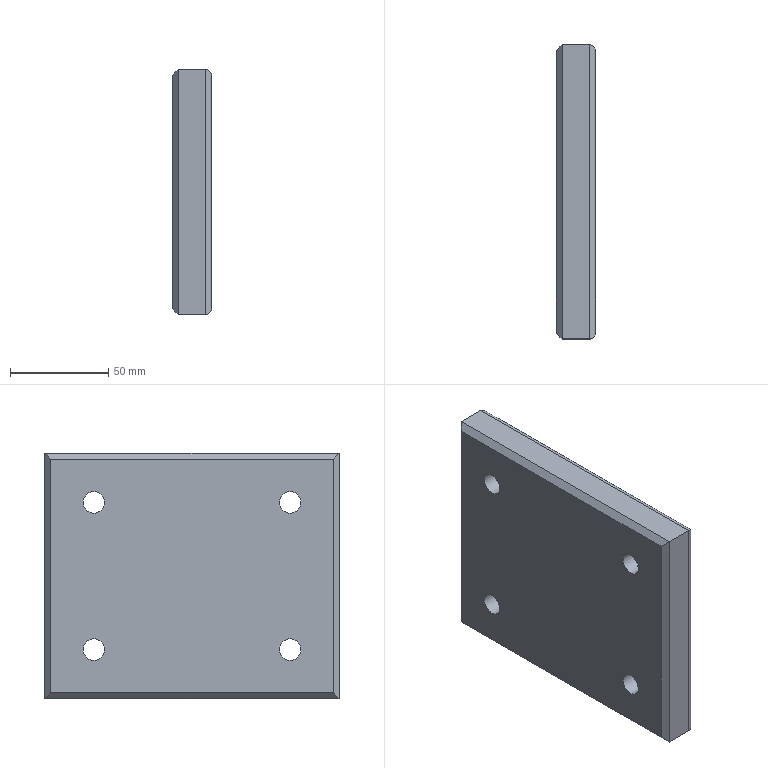Part | NX | features solid 2 | 1 solid | 26 faces | box 20 x 150 x 125 mm | volume 356923 mm3 | plane 14 | cylinder 12 | commonest cylinder face diameters 6 x4 11 x4 17.5 x4
STEP:
#1=CARTESIAN_POINT('',(803.,75.,-130.));
#2=VERTEX_POINT('',#1);
#3=CARTESIAN_POINT('',(817.,75.,-130.));
#4=VERTEX_POINT('',#3);
#5=CARTESIAN_POINT('',(800.,75.,-130.));
#6=DIRECTION('',(1.,0.,0.));
#7=VECTOR('',#6,1000.);
#8=LINE('',#5,#7);
#9=EDGE_CURVE('',#2,#4,#8,.T.);
#10=ORIENTED_EDGE('',*,*,#9,.T.);
#11=CARTESIAN_POINT('',(817.,-75.,-130.));
#12=VERTEX_POINT('',#11);
#13=CARTESIAN_POINT('',(817.,50.,-130.));
#14=DIRECTION('',(0.,1.,0.));
#15=VECTOR('',#14,1000.);
#16=LINE('',#13,#15);
#17=EDGE_CURVE('',#12,#4,#16,.T.);
#18=ORIENTED_EDGE('',*,*,#17,.F.);
#19=CARTESIAN_POINT('',(803.,-75.,-130.));
#20=VERTEX_POINT('',#19);
#21=CARTESIAN_POINT('',(800.,-75.,-130.));
#22=DIRECTION('',(1.,0.,0.));
#23=VECTOR('',#22,1000.);
#24=LINE('',#21,#23);
#25=EDGE_CURVE('',#20,#12,#24,.T.);
#26=ORIENTED_EDGE('',*,*,#25,.F.);
#27=CARTESIAN_POINT('',(803.,-50.,-130.));
#28=DIRECTION('',(0.,-1.,0.));
#29=VECTOR('',#28,1000.);
#30=LINE('',#27,#29);
#31=EDGE_CURVE('',#2,#20,#30,.T.);
#32=ORIENTED_EDGE('',*,*,#31,.F.);
#33=EDGE_LOOP('',(#10,#18,#26,#32));
#34=FACE_BOUND('',#33,.T.);
#35=CARTESIAN_POINT('',(800.,-50.,-130.));
#36=DIRECTION('',(0.,0.,1.));
#37=DIRECTION('',(0.,-1.,0.));
#38=AXIS2_PLACEMENT_3D('',#35,#36,#37);
#39=PLANE('',#38);
#40=ADVANCED_FACE('',(#34),#39,.F.);
#41=CARTESIAN_POINT('',(803.,75.,-5.));
#42=VERTEX_POINT('',#41);
#43=CARTESIAN_POINT('',(817.,75.,-5.));
#44=VERTEX_POINT('',#43);
#45=CARTESIAN_POINT('',(800.,75.,-5.));
#46=DIRECTION('',(1.,0.,0.));
#47=VECTOR('',#46,1000.);
#48=LINE('',#45,#47);
#49=EDGE_CURVE('',#42,#44,#48,.T.);
#50=ORIENTED_EDGE('',*,*,#49,.T.);
#51=CARTESIAN_POINT('',(817.,75.,-5.));
#52=DIRECTION('',(0.,0.,1.));
#53=VECTOR('',#52,1000.);
#54=LINE('',#51,#53);
#55=EDGE_CURVE('',#4,#44,#54,.T.);
#56=ORIENTED_EDGE('',*,*,#55,.F.);
#57=ORIENTED_EDGE('',*,*,#9,.F.);
#58=CARTESIAN_POINT('',(803.,75.,-105.));
#59=DIRECTION('',(0.,0.,-1.));
#60=VECTOR('',#59,1000.);
#61=LINE('',#58,#60);
#62=EDGE_CURVE('',#42,#2,#61,.T.);
#63=ORIENTED_EDGE('',*,*,#62,.F.);
#64=EDGE_LOOP('',(#50,#56,#57,#63));
#65=FACE_BOUND('',#64,.T.);
#66=CARTESIAN_POINT('',(800.,75.,-105.));
#67=DIRECTION('',(0.,-1.,0.));
#68=DIRECTION('',(-1.,0.,0.));
#69=AXIS2_PLACEMENT_3D('',#66,#67,#68);
#70=PLANE('',#69);
#71=ADVANCED_FACE('',(#65),#70,.F.);
#72=CARTESIAN_POINT('',(803.,-75.,-5.));
#73=VERTEX_POINT('',#72);
#74=CARTESIAN_POINT('',(817.,-75.,-5.));
#75=VERTEX_POINT('',#74);
#76=CARTESIAN_POINT('',(800.,-75.,-5.));
#77=DIRECTION('',(1.,0.,0.));
#78=VECTOR('',#77,1000.);
#79=LINE('',#76,#78);
#80=EDGE_CURVE('',#73,#75,#79,.T.);
#81=ORIENTED_EDGE('',*,*,#80,.T.);
#82=CARTESIAN_POINT('',(817.,-50.,-5.));
#83=DIRECTION('',(0.,-1.,0.));
#84=VECTOR('',#83,1000.);
#85=LINE('',#82,#84);
#86=EDGE_CURVE('',#44,#75,#85,.T.);
#87=ORIENTED_EDGE('',*,*,#86,.F.);
#88=ORIENTED_EDGE('',*,*,#49,.F.);
#89=CARTESIAN_POINT('',(803.,50.,-5.));
#90=DIRECTION('',(0.,1.,0.));
#91=VECTOR('',#90,1000.);
#92=LINE('',#89,#91);
#93=EDGE_CURVE('',#73,#42,#92,.T.);
#94=ORIENTED_EDGE('',*,*,#93,.F.);
#95=EDGE_LOOP('',(#81,#87,#88,#94));
#96=FACE_BOUND('',#95,.T.);
#97=CARTESIAN_POINT('',(800.,50.,-5.));
#98=DIRECTION('',(0.,0.,-1.));
#99=DIRECTION('',(-1.,0.,0.));
#100=AXIS2_PLACEMENT_3D('',#97,#98,#99);
#101=PLANE('',#100);
#102=ADVANCED_FACE('',(#96),#101,.F.);
#103=ORIENTED_EDGE('',*,*,#25,.T.);
#104=CARTESIAN_POINT('',(817.,-75.,-105.));
#105=DIRECTION('',(0.,0.,-1.));
#106=VECTOR('',#105,1000.);
#107=LINE('',#104,#106);
#108=EDGE_CURVE('',#75,#12,#107,.T.);
#109=ORIENTED_EDGE('',*,*,#108,.F.);
#110=ORIENTED_EDGE('',*,*,#80,.F.);
#111=CARTESIAN_POINT('',(803.,-75.,-5.));
#112=DIRECTION('',(0.,0.,1.));
#113=VECTOR('',#112,1000.);
#114=LINE('',#111,#113);
#115=EDGE_CURVE('',#20,#73,#114,.T.);
#116=ORIENTED_EDGE('',*,*,#115,.F.);
#117=EDGE_LOOP('',(#103,#109,#110,#116));
#118=FACE_BOUND('',#117,.T.);
#119=CARTESIAN_POINT('',(800.,-75.,-5.));
#120=DIRECTION('',(0.,1.,0.));
#121=DIRECTION('',(0.,0.,1.));
#122=AXIS2_PLACEMENT_3D('',#119,#120,#121);
#123=PLANE('',#122);
#124=ADVANCED_FACE('',(#118),#123,.F.);
#125=CARTESIAN_POINT('',(800.,72.,-127.));
#126=VERTEX_POINT('',#125);
#127=CARTESIAN_POINT('',(800.,72.,-8.));
#128=VERTEX_POINT('',#127);
#129=CARTESIAN_POINT('',(800.,72.,-105.));
#130=DIRECTION('',(0.,0.,1.));
#131=VECTOR('',#130,1000.);
#132=LINE('',#129,#131);
#133=EDGE_CURVE('',#126,#128,#132,.T.);
#134=ORIENTED_EDGE('',*,*,#133,.F.);
#135=CARTESIAN_POINT('',(800.,-72.,-127.));
#136=VERTEX_POINT('',#135);
#137=CARTESIAN_POINT('',(800.,-50.,-127.));
#138=DIRECTION('',(0.,1.,0.));
#139=VECTOR('',#138,1000.);
#140=LINE('',#137,#139);
#141=EDGE_CURVE('',#136,#126,#140,.T.);
#142=ORIENTED_EDGE('',*,*,#141,.F.);
#143=CARTESIAN_POINT('',(800.,-72.,-8.));
#144=VERTEX_POINT('',#143);
#145=CARTESIAN_POINT('',(800.,-72.,-105.));
#146=DIRECTION('',(0.,0.,-1.));
#147=VECTOR('',#146,1000.);
#148=LINE('',#145,#147);
#149=EDGE_CURVE('',#144,#136,#148,.T.);
#150=ORIENTED_EDGE('',*,*,#149,.F.);
#151=CARTESIAN_POINT('',(800.,-50.,-8.));
#152=DIRECTION('',(0.,-1.,0.));
#153=VECTOR('',#152,1000.);
#154=LINE('',#151,#153);
#155=EDGE_CURVE('',#128,#144,#154,.T.);
#156=ORIENTED_EDGE('',*,*,#155,.F.);
#157=EDGE_LOOP('',(#134,#142,#150,#156));
#158=FACE_BOUND('',#157,.T.);
#159=CARTESIAN_POINT('',(800.,50.,-35.5));
#160=VERTEX_POINT('',#159);
#161=CARTESIAN_POINT('',(800.,50.,-30.));
#162=DIRECTION('',(-1.,0.,0.));
#163=DIRECTION('',(0.,0.,-1.));
#164=AXIS2_PLACEMENT_3D('',#161,#162,#163);
#165=CIRCLE('',#164,5.5);
#166=EDGE_CURVE('',#160,#160,#165,.T.);
#167=ORIENTED_EDGE('',*,*,#166,.F.);
#168=EDGE_LOOP('',(#167));
#169=FACE_BOUND('',#168,.T.);
#170=CARTESIAN_POINT('',(800.,-50.,-35.5));
#171=VERTEX_POINT('',#170);
#172=CARTESIAN_POINT('',(800.,-50.,-30.));
#173=DIRECTION('',(-1.,0.,0.));
#174=DIRECTION('',(0.,0.,-1.));
#175=AXIS2_PLACEMENT_3D('',#172,#173,#174);
#176=CIRCLE('',#175,5.5);
#177=EDGE_CURVE('',#171,#171,#176,.T.);
#178=ORIENTED_EDGE('',*,*,#177,.F.);
#179=EDGE_LOOP('',(#178));
#180=FACE_BOUND('',#179,.T.);
#181=CARTESIAN_POINT('',(800.,50.,-110.5));
#182=VERTEX_POINT('',#181);
#183=CARTESIAN_POINT('',(800.,50.,-105.));
#184=DIRECTION('',(-1.,0.,0.));
#185=DIRECTION('',(0.,0.,-1.));
#186=AXIS2_PLACEMENT_3D('',#183,#184,#185);
#187=CIRCLE('',#186,5.5);
#188=EDGE_CURVE('',#182,#182,#187,.T.);
#189=ORIENTED_EDGE('',*,*,#188,.F.);
#190=EDGE_LOOP('',(#189));
#191=FACE_BOUND('',#190,.T.);
#192=CARTESIAN_POINT('',(800.,-50.,-110.5));
#193=VERTEX_POINT('',#192);
#194=CARTESIAN_POINT('',(800.,-50.,-105.));
#195=DIRECTION('',(-1.,0.,0.));
#196=DIRECTION('',(0.,0.,-1.));
#197=AXIS2_PLACEMENT_3D('',#194,#195,#196);
#198=CIRCLE('',#197,5.5);
#199=EDGE_CURVE('',#193,#193,#198,.T.);
#200=ORIENTED_EDGE('',*,*,#199,.F.);
#201=EDGE_LOOP('',(#200));
#202=FACE_BOUND('',#201,.T.);
#203=CARTESIAN_POINT('',(800.,-50.,-105.));
#204=DIRECTION('',(1.,0.,0.));
#205=DIRECTION('',(0.,0.,-1.));
#206=AXIS2_PLACEMENT_3D('',#203,#204,#205);
#207=PLANE('',#206);
#208=ADVANCED_FACE('',(#158,#169,#180,#191,#202),#207,.F.);
#209=CARTESIAN_POINT('',(820.,72.,-127.));
#210=VERTEX_POINT('',#209);
#211=CARTESIAN_POINT('',(820.,-72.,-127.));
#212=VERTEX_POINT('',#211);
#213=CARTESIAN_POINT('',(820.,-50.,-127.));
#214=DIRECTION('',(0.,1.,0.));
#215=VECTOR('',#214,1000.);
#216=LINE('',#213,#215);
#217=EDGE_CURVE('',#210,#212,#216,.F.);
#218=ORIENTED_EDGE('',*,*,#217,.F.);
#219=CARTESIAN_POINT('',(820.,72.,-8.));
#220=VERTEX_POINT('',#219);
#221=CARTESIAN_POINT('',(820.,72.,-105.));
#222=DIRECTION('',(0.,0.,1.));
#223=VECTOR('',#222,1000.);
#224=LINE('',#221,#223);
#225=EDGE_CURVE('',#220,#210,#224,.F.);
#226=ORIENTED_EDGE('',*,*,#225,.F.);
#227=CARTESIAN_POINT('',(820.,-72.,-8.));
#228=VERTEX_POINT('',#227);
#229=CARTESIAN_POINT('',(820.,50.,-8.));
#230=DIRECTION('',(0.,-1.,0.));
#231=VECTOR('',#230,1000.);
#232=LINE('',#229,#231);
#233=EDGE_CURVE('',#228,#220,#232,.F.);
#234=ORIENTED_EDGE('',*,*,#233,.F.);
#235=CARTESIAN_POINT('',(820.,-72.,-5.));
#236=DIRECTION('',(0.,0.,-1.));
#237=VECTOR('',#236,1000.);
#238=LINE('',#235,#237);
#239=EDGE_CURVE('',#212,#228,#238,.F.);
#240=ORIENTED_EDGE('',*,*,#239,.F.);
#241=EDGE_LOOP('',(#218,#226,#234,#240));
#242=FACE_BOUND('',#241,.T.);
#243=CARTESIAN_POINT('',(820.,50.,-21.25));
#244=VERTEX_POINT('',#243);
#245=CARTESIAN_POINT('',(820.,50.,-30.));
#246=DIRECTION('',(1.,0.,0.));
#247=DIRECTION('',(0.,0.,1.));
#248=AXIS2_PLACEMENT_3D('',#245,#246,#247);
#249=CIRCLE('',#248,8.75);
#250=EDGE_CURVE('',#244,#244,#249,.T.);
#251=ORIENTED_EDGE('',*,*,#250,.F.);
#252=EDGE_LOOP('',(#251));
#253=FACE_BOUND('',#252,.T.);
#254=CARTESIAN_POINT('',(820.,-50.,-21.25));
#255=VERTEX_POINT('',#254);
#256=CARTESIAN_POINT('',(820.,-50.,-30.));
#257=DIRECTION('',(1.,0.,0.));
#258=DIRECTION('',(0.,0.,1.));
#259=AXIS2_PLACEMENT_3D('',#256,#257,#258);
#260=CIRCLE('',#259,8.75);
#261=EDGE_CURVE('',#255,#255,#260,.T.);
#262=ORIENTED_EDGE('',*,*,#261,.F.);
#263=EDGE_LOOP('',(#262));
#264=FACE_BOUND('',#263,.T.);
#265=CARTESIAN_POINT('',(820.,50.,-96.25));
#266=VERTEX_POINT('',#265);
#267=CARTESIAN_POINT('',(820.,50.,-105.));
#268=DIRECTION('',(1.,0.,0.));
#269=DIRECTION('',(0.,0.,1.));
#270=AXIS2_PLACEMENT_3D('',#267,#268,#269);
#271=CIRCLE('',#270,8.75);
#272=EDGE_CURVE('',#266,#266,#271,.T.);
#273=ORIENTED_EDGE('',*,*,#272,.F.);
#274=EDGE_LOOP('',(#273));
#275=FACE_BOUND('',#274,.T.);
#276=CARTESIAN_POINT('',(820.,-50.,-96.25));
#277=VERTEX_POINT('',#276);
#278=CARTESIAN_POINT('',(820.,-50.,-105.));
#279=DIRECTION('',(1.,0.,0.));
#280=DIRECTION('',(0.,0.,1.));
#281=AXIS2_PLACEMENT_3D('',#278,#279,#280);
#282=CIRCLE('',#281,8.75);
#283=EDGE_CURVE('',#277,#277,#282,.T.);
#284=ORIENTED_EDGE('',*,*,#283,.F.);
#285=EDGE_LOOP('',(#284));
#286=FACE_BOUND('',#285,.T.);
#287=CARTESIAN_POINT('',(820.,-50.,-105.));
#288=DIRECTION('',(1.,0.,0.));
#289=DIRECTION('',(0.,0.,-1.));
#290=AXIS2_PLACEMENT_3D('',#287,#288,#289);
#291=PLANE('',#290);
#292=ADVANCED_FACE('',(#242,#253,#264,#275,#286),#291,.T.);
#293=CARTESIAN_POINT('',(808.,-50.,-99.5));
#294=VERTEX_POINT('',#293);
#295=CARTESIAN_POINT('',(808.,-50.,-105.));
#296=DIRECTION('',(1.,0.,0.));
#297=DIRECTION('',(0.,0.,1.));
#298=AXIS2_PLACEMENT_3D('',#295,#296,#297);
#299=CIRCLE('',#298,5.5);
#300=EDGE_CURVE('',#294,#294,#299,.T.);
#301=ORIENTED_EDGE('',*,*,#300,.T.);
#302=EDGE_LOOP('',(#301));
#303=FACE_BOUND('',#302,.T.);
#304=ORIENTED_EDGE('',*,*,#199,.T.);
#305=EDGE_LOOP('',(#304));
#306=FACE_BOUND('',#305,.T.);
#307=CARTESIAN_POINT('',(770.,-50.,-105.));
#308=DIRECTION('',(-1.,0.,0.));
#309=DIRECTION('',(0.,0.,1.));
#310=AXIS2_PLACEMENT_3D('',#307,#308,#309);
#311=CYLINDRICAL_SURFACE('',#310,5.5);
#312=ADVANCED_FACE('',(#303,#306),#311,.F.);
#313=ORIENTED_EDGE('',*,*,#300,.F.);
#314=EDGE_LOOP('',(#313));
#315=FACE_BOUND('',#314,.T.);
#316=CARTESIAN_POINT('',(808.,-50.,-96.25));
#317=VERTEX_POINT('',#316);
#318=CARTESIAN_POINT('',(808.,-50.,-105.));
#319=DIRECTION('',(1.,0.,0.));
#320=DIRECTION('',(0.,0.,1.));
#321=AXIS2_PLACEMENT_3D('',#318,#319,#320);
#322=CIRCLE('',#321,8.75);
#323=EDGE_CURVE('',#317,#317,#322,.T.);
#324=ORIENTED_EDGE('',*,*,#323,.T.);
#325=EDGE_LOOP('',(#324));
#326=FACE_BOUND('',#325,.T.);
#327=CARTESIAN_POINT('',(808.,-50.,-105.));
#328=DIRECTION('',(-1.,0.,0.));
#329=DIRECTION('',(0.,0.,1.));
#330=AXIS2_PLACEMENT_3D('',#327,#328,#329);
#331=PLANE('',#330);
#332=ADVANCED_FACE('',(#315,#326),#331,.F.);
#333=ORIENTED_EDGE('',*,*,#323,.F.);
#334=EDGE_LOOP('',(#333));
#335=FACE_BOUND('',#334,.T.);
#336=ORIENTED_EDGE('',*,*,#283,.T.);
#337=EDGE_LOOP('',(#336));
#338=FACE_BOUND('',#337,.T.);
#339=CARTESIAN_POINT('',(820.,-50.,-105.));
#340=DIRECTION('',(-1.,0.,0.));
#341=DIRECTION('',(0.,0.,1.));
#342=AXIS2_PLACEMENT_3D('',#339,#340,#341);
#343=CYLINDRICAL_SURFACE('',#342,8.75);
#344=ADVANCED_FACE('',(#335,#338),#343,.F.);
#345=CARTESIAN_POINT('',(808.,50.,-99.5));
#346=VERTEX_POINT('',#345);
#347=CARTESIAN_POINT('',(808.,50.,-105.));
#348=DIRECTION('',(1.,0.,0.));
#349=DIRECTION('',(0.,0.,1.));
#350=AXIS2_PLACEMENT_3D('',#347,#348,#349);
#351=CIRCLE('',#350,5.5);
#352=EDGE_CURVE('',#346,#346,#351,.T.);
#353=ORIENTED_EDGE('',*,*,#352,.T.);
#354=EDGE_LOOP('',(#353));
#355=FACE_BOUND('',#354,.T.);
#356=ORIENTED_EDGE('',*,*,#188,.T.);
#357=EDGE_LOOP('',(#356));
#358=FACE_BOUND('',#357,.T.);
#359=CARTESIAN_POINT('',(770.,50.,-105.));
#360=DIRECTION('',(-1.,0.,0.));
#361=DIRECTION('',(0.,0.,1.));
#362=AXIS2_PLACEMENT_3D('',#359,#360,#361);
#363=CYLINDRICAL_SURFACE('',#362,5.5);
#364=ADVANCED_FACE('',(#355,#358),#363,.F.);
#365=ORIENTED_EDGE('',*,*,#352,.F.);
#366=EDGE_LOOP('',(#365));
#367=FACE_BOUND('',#366,.T.);
#368=CARTESIAN_POINT('',(808.,50.,-96.25));
#369=VERTEX_POINT('',#368);
#370=CARTESIAN_POINT('',(808.,50.,-105.));
#371=DIRECTION('',(1.,0.,0.));
#372=DIRECTION('',(0.,0.,1.));
#373=AXIS2_PLACEMENT_3D('',#370,#371,#372);
#374=CIRCLE('',#373,8.75);
#375=EDGE_CURVE('',#369,#369,#374,.T.);
#376=ORIENTED_EDGE('',*,*,#375,.T.);
#377=EDGE_LOOP('',(#376));
#378=FACE_BOUND('',#377,.T.);
#379=CARTESIAN_POINT('',(808.,50.,-105.));
#380=DIRECTION('',(-1.,0.,0.));
#381=DIRECTION('',(0.,0.,1.));
#382=AXIS2_PLACEMENT_3D('',#379,#380,#381);
#383=PLANE('',#382);
#384=ADVANCED_FACE('',(#367,#378),#383,.F.);
#385=ORIENTED_EDGE('',*,*,#375,.F.);
#386=EDGE_LOOP('',(#385));
#387=FACE_BOUND('',#386,.T.);
#388=ORIENTED_EDGE('',*,*,#272,.T.);
#389=EDGE_LOOP('',(#388));
#390=FACE_BOUND('',#389,.T.);
#391=CARTESIAN_POINT('',(820.,50.,-105.));
#392=DIRECTION('',(-1.,0.,0.));
#393=DIRECTION('',(0.,0.,1.));
#394=AXIS2_PLACEMENT_3D('',#391,#392,#393);
#395=CYLINDRICAL_SURFACE('',#394,8.75);
#396=ADVANCED_FACE('',(#387,#390),#395,.F.);
#397=CARTESIAN_POINT('',(808.,-50.,-24.5));
#398=VERTEX_POINT('',#397);
#399=CARTESIAN_POINT('',(808.,-50.,-30.));
#400=DIRECTION('',(1.,0.,0.));
#401=DIRECTION('',(0.,0.,1.));
#402=AXIS2_PLACEMENT_3D('',#399,#400,#401);
#403=CIRCLE('',#402,5.5);
#404=EDGE_CURVE('',#398,#398,#403,.T.);
#405=ORIENTED_EDGE('',*,*,#404,.T.);
#406=EDGE_LOOP('',(#405));
#407=FACE_BOUND('',#406,.T.);
#408=ORIENTED_EDGE('',*,*,#177,.T.);
#409=EDGE_LOOP('',(#408));
#410=FACE_BOUND('',#409,.T.);
#411=CARTESIAN_POINT('',(770.,-50.,-30.));
#412=DIRECTION('',(-1.,0.,0.));
#413=DIRECTION('',(0.,0.,1.));
#414=AXIS2_PLACEMENT_3D('',#411,#412,#413);
#415=CYLINDRICAL_SURFACE('',#414,5.5);
#416=ADVANCED_FACE('',(#407,#410),#415,.F.);
#417=ORIENTED_EDGE('',*,*,#404,.F.);
#418=EDGE_LOOP('',(#417));
#419=FACE_BOUND('',#418,.T.);
#420=CARTESIAN_POINT('',(808.,-50.,-21.25));
#421=VERTEX_POINT('',#420);
#422=CARTESIAN_POINT('',(808.,-50.,-30.));
#423=DIRECTION('',(1.,0.,0.));
#424=DIRECTION('',(0.,0.,1.));
#425=AXIS2_PLACEMENT_3D('',#422,#423,#424);
#426=CIRCLE('',#425,8.75);
#427=EDGE_CURVE('',#421,#421,#426,.T.);
#428=ORIENTED_EDGE('',*,*,#427,.T.);
#429=EDGE_LOOP('',(#428));
#430=FACE_BOUND('',#429,.T.);
#431=CARTESIAN_POINT('',(808.,-50.,-30.));
#432=DIRECTION('',(-1.,0.,0.));
#433=DIRECTION('',(0.,0.,1.));
#434=AXIS2_PLACEMENT_3D('',#431,#432,#433);
#435=PLANE('',#434);
#436=ADVANCED_FACE('',(#419,#430),#435,.F.);
#437=ORIENTED_EDGE('',*,*,#427,.F.);
#438=EDGE_LOOP('',(#437));
#439=FACE_BOUND('',#438,.T.);
#440=ORIENTED_EDGE('',*,*,#261,.T.);
#441=EDGE_LOOP('',(#440));
#442=FACE_BOUND('',#441,.T.);
#443=CARTESIAN_POINT('',(820.,-50.,-30.));
#444=DIRECTION('',(-1.,0.,0.));
#445=DIRECTION('',(0.,0.,1.));
#446=AXIS2_PLACEMENT_3D('',#443,#444,#445);
#447=CYLINDRICAL_SURFACE('',#446,8.75);
#448=ADVANCED_FACE('',(#439,#442),#447,.F.);
#449=CARTESIAN_POINT('',(808.,50.,-24.5));
#450=VERTEX_POINT('',#449);
#451=CARTESIAN_POINT('',(808.,50.,-30.));
#452=DIRECTION('',(1.,0.,0.));
#453=DIRECTION('',(0.,0.,1.));
#454=AXIS2_PLACEMENT_3D('',#451,#452,#453);
#455=CIRCLE('',#454,5.5);
#456=EDGE_CURVE('',#450,#450,#455,.T.);
#457=ORIENTED_EDGE('',*,*,#456,.T.);
#458=EDGE_LOOP('',(#457));
#459=FACE_BOUND('',#458,.T.);
#460=ORIENTED_EDGE('',*,*,#166,.T.);
#461=EDGE_LOOP('',(#460));
#462=FACE_BOUND('',#461,.T.);
#463=CARTESIAN_POINT('',(770.,50.,-30.));
#464=DIRECTION('',(-1.,0.,0.));
#465=DIRECTION('',(0.,0.,1.));
#466=AXIS2_PLACEMENT_3D('',#463,#464,#465);
#467=CYLINDRICAL_SURFACE('',#466,5.5);
#468=ADVANCED_FACE('',(#459,#462),#467,.F.);
#469=ORIENTED_EDGE('',*,*,#456,.F.);
#470=EDGE_LOOP('',(#469));
#471=FACE_BOUND('',#470,.T.);
#472=CARTESIAN_POINT('',(808.,50.,-21.25));
#473=VERTEX_POINT('',#472);
#474=CARTESIAN_POINT('',(808.,50.,-30.));
#475=DIRECTION('',(1.,0.,0.));
#476=DIRECTION('',(0.,0.,1.));
#477=AXIS2_PLACEMENT_3D('',#474,#475,#476);
#478=CIRCLE('',#477,8.75);
#479=EDGE_CURVE('',#473,#473,#478,.T.);
#480=ORIENTED_EDGE('',*,*,#479,.T.);
#481=EDGE_LOOP('',(#480));
#482=FACE_BOUND('',#481,.T.);
#483=CARTESIAN_POINT('',(808.,50.,-30.));
#484=DIRECTION('',(-1.,0.,0.));
#485=DIRECTION('',(0.,0.,1.));
#486=AXIS2_PLACEMENT_3D('',#483,#484,#485);
#487=PLANE('',#486);
#488=ADVANCED_FACE('',(#471,#482),#487,.F.);
#489=ORIENTED_EDGE('',*,*,#479,.F.);
#490=EDGE_LOOP('',(#489));
#491=FACE_BOUND('',#490,.T.);
#492=ORIENTED_EDGE('',*,*,#250,.T.);
#493=EDGE_LOOP('',(#492));
#494=FACE_BOUND('',#493,.T.);
#495=CARTESIAN_POINT('',(820.,50.,-30.));
#496=DIRECTION('',(-1.,0.,0.));
#497=DIRECTION('',(0.,0.,1.));
#498=AXIS2_PLACEMENT_3D('',#495,#496,#497);
#499=CYLINDRICAL_SURFACE('',#498,8.75);
#500=ADVANCED_FACE('',(#491,#494),#499,.F.);
#501=CARTESIAN_POINT('',(817.,72.,-127.));
#502=DIRECTION('',(0.,0.7071,0.7071));
#503=DIRECTION('',(0.,-0.7071,0.7071));
#504=AXIS2_PLACEMENT_3D('',#501,#502,#503);
#505=ELLIPSE('',#504,4.243,3.);
#506=EDGE_CURVE('',#210,#4,#505,.T.);
#507=ORIENTED_EDGE('',*,*,#506,.T.);
#508=ORIENTED_EDGE('',*,*,#55,.T.);
#509=CARTESIAN_POINT('',(817.,72.,-8.));
#510=DIRECTION('',(0.,-0.7071,0.7071));
#511=DIRECTION('',(0.,-0.7071,-0.7071));
#512=AXIS2_PLACEMENT_3D('',#509,#510,#511);
#513=ELLIPSE('',#512,4.243,3.);
#514=EDGE_CURVE('',#44,#220,#513,.F.);
#515=ORIENTED_EDGE('',*,*,#514,.T.);
#516=ORIENTED_EDGE('',*,*,#225,.T.);
#517=EDGE_LOOP('',(#507,#508,#515,#516));
#518=FACE_BOUND('',#517,.T.);
#519=CARTESIAN_POINT('',(817.,72.,-105.));
#520=DIRECTION('',(0.,0.,-1.));
#521=DIRECTION('',(-1.,0.,0.));
#522=AXIS2_PLACEMENT_3D('',#519,#520,#521);
#523=CYLINDRICAL_SURFACE('',#522,3.);
#524=ADVANCED_FACE('',(#518),#523,.T.);
#525=ORIENTED_EDGE('',*,*,#514,.F.);
#526=ORIENTED_EDGE('',*,*,#86,.T.);
#527=CARTESIAN_POINT('',(817.,-72.,-8.));
#528=DIRECTION('',(0.,-0.7071,-0.7071));
#529=DIRECTION('',(0.,0.7071,-0.7071));
#530=AXIS2_PLACEMENT_3D('',#527,#528,#529);
#531=ELLIPSE('',#530,4.243,3.);
#532=EDGE_CURVE('',#75,#228,#531,.F.);
#533=ORIENTED_EDGE('',*,*,#532,.T.);
#534=ORIENTED_EDGE('',*,*,#233,.T.);
#535=EDGE_LOOP('',(#525,#526,#533,#534));
#536=FACE_BOUND('',#535,.T.);
#537=CARTESIAN_POINT('',(817.,50.,-8.));
#538=DIRECTION('',(0.,1.,0.));
#539=DIRECTION('',(1.,0.,0.));
#540=AXIS2_PLACEMENT_3D('',#537,#538,#539);
#541=CYLINDRICAL_SURFACE('',#540,3.);
#542=ADVANCED_FACE('',(#536),#541,.T.);
#543=ORIENTED_EDGE('',*,*,#506,.F.);
#544=ORIENTED_EDGE('',*,*,#217,.T.);
#545=CARTESIAN_POINT('',(817.,-72.,-127.));
#546=DIRECTION('',(0.,0.7071,-0.7071));
#547=DIRECTION('',(0.,-0.7071,-0.7071));
#548=AXIS2_PLACEMENT_3D('',#545,#546,#547);
#549=ELLIPSE('',#548,4.243,3.);
#550=EDGE_CURVE('',#212,#12,#549,.T.);
#551=ORIENTED_EDGE('',*,*,#550,.T.);
#552=ORIENTED_EDGE('',*,*,#17,.T.);
#553=EDGE_LOOP('',(#543,#544,#551,#552));
#554=FACE_BOUND('',#553,.T.);
#555=CARTESIAN_POINT('',(817.,-50.,-127.));
#556=DIRECTION('',(0.,-1.,0.));
#557=DIRECTION('',(0.,0.,-1.));
#558=AXIS2_PLACEMENT_3D('',#555,#556,#557);
#559=CYLINDRICAL_SURFACE('',#558,3.);
#560=ADVANCED_FACE('',(#554),#559,.T.);
#561=ORIENTED_EDGE('',*,*,#532,.F.);
#562=ORIENTED_EDGE('',*,*,#108,.T.);
#563=ORIENTED_EDGE('',*,*,#550,.F.);
#564=ORIENTED_EDGE('',*,*,#239,.T.);
#565=EDGE_LOOP('',(#561,#562,#563,#564));
#566=FACE_BOUND('',#565,.T.);
#567=CARTESIAN_POINT('',(817.,-72.,-5.));
#568=DIRECTION('',(0.,0.,1.));
#569=DIRECTION('',(0.,-1.,0.));
#570=AXIS2_PLACEMENT_3D('',#567,#568,#569);
#571=CYLINDRICAL_SURFACE('',#570,3.);
#572=ADVANCED_FACE('',(#566),#571,.T.);
#573=CARTESIAN_POINT('',(801.,-73.,-128.));
#574=DIRECTION('',(-0.5774,0.5774,0.5774));
#575=VECTOR('',#574,1000.);
#576=LINE('',#573,#575);
#577=EDGE_CURVE('',#20,#136,#576,.T.);
#578=ORIENTED_EDGE('',*,*,#577,.T.);
#579=ORIENTED_EDGE('',*,*,#141,.T.);
#580=CARTESIAN_POINT('',(767.667,39.667,-94.667));
#581=DIRECTION('',(-0.5774,-0.5774,0.5774));
#582=VECTOR('',#581,1000.);
#583=LINE('',#580,#582);
#584=EDGE_CURVE('',#126,#2,#583,.F.);
#585=ORIENTED_EDGE('',*,*,#584,.T.);
#586=ORIENTED_EDGE('',*,*,#31,.T.);
#587=EDGE_LOOP('',(#578,#579,#585,#586));
#588=FACE_BOUND('',#587,.T.);
#589=CARTESIAN_POINT('',(800.,-50.,-127.));
#590=DIRECTION('',(0.7071,0.,0.7071));
#591=DIRECTION('',(0.7071,0.,-0.7071));
#592=AXIS2_PLACEMENT_3D('',#589,#590,#591);
#593=PLANE('',#592);
#594=ADVANCED_FACE('',(#588),#593,.F.);
#595=ORIENTED_EDGE('',*,*,#584,.F.);
#596=ORIENTED_EDGE('',*,*,#133,.T.);
#597=CARTESIAN_POINT('',(767.667,39.667,-40.333));
#598=DIRECTION('',(-0.5774,-0.5774,-0.5774));
#599=VECTOR('',#598,1000.);
#600=LINE('',#597,#599);
#601=EDGE_CURVE('',#128,#42,#600,.F.);
#602=ORIENTED_EDGE('',*,*,#601,.T.);
#603=ORIENTED_EDGE('',*,*,#62,.T.);
#604=EDGE_LOOP('',(#595,#596,#602,#603));
#605=FACE_BOUND('',#604,.T.);
#606=CARTESIAN_POINT('',(800.,72.,-105.));
#607=DIRECTION('',(0.7071,-0.7071,0.));
#608=DIRECTION('',(-0.7071,-0.7071,0.));
#609=AXIS2_PLACEMENT_3D('',#606,#607,#608);
#610=PLANE('',#609);
#611=ADVANCED_FACE('',(#605),#610,.F.);
#612=ORIENTED_EDGE('',*,*,#577,.F.);
#613=ORIENTED_EDGE('',*,*,#115,.T.);
#614=CARTESIAN_POINT('',(767.667,-39.667,-40.333));
#615=DIRECTION('',(0.5774,-0.5774,0.5774));
#616=VECTOR('',#615,1000.);
#617=LINE('',#614,#616);
#618=EDGE_CURVE('',#73,#144,#617,.F.);
#619=ORIENTED_EDGE('',*,*,#618,.T.);
#620=ORIENTED_EDGE('',*,*,#149,.T.);
#621=EDGE_LOOP('',(#612,#613,#619,#620));
#622=FACE_BOUND('',#621,.T.);
#623=CARTESIAN_POINT('',(800.,-72.,-105.));
#624=DIRECTION('',(0.7071,0.7071,0.));
#625=DIRECTION('',(0.7071,-0.7071,0.));
#626=AXIS2_PLACEMENT_3D('',#623,#624,#625);
#627=PLANE('',#626);
#628=ADVANCED_FACE('',(#622),#627,.F.);
#629=ORIENTED_EDGE('',*,*,#601,.F.);
#630=ORIENTED_EDGE('',*,*,#155,.T.);
#631=ORIENTED_EDGE('',*,*,#618,.F.);
#632=ORIENTED_EDGE('',*,*,#93,.T.);
#633=EDGE_LOOP('',(#629,#630,#631,#632));
#634=FACE_BOUND('',#633,.T.);
#635=CARTESIAN_POINT('',(800.,-50.,-8.));
#636=DIRECTION('',(0.7071,0.,-0.7071));
#637=DIRECTION('',(-0.7071,0.,-0.7071));
#638=AXIS2_PLACEMENT_3D('',#635,#636,#637);
#639=PLANE('',#638);
#640=ADVANCED_FACE('',(#634),#639,.F.);
#641=CLOSED_SHELL('',(#40,#71,#102,#124,#208,#292,#312,#332,#344,#364,#384,#396,#416,#436,#448,#468,#488,#500,#524,#542,#560,#572,#594,#611,#628,#640));
#642=MANIFOLD_SOLID_BREP('',#641);
#643=(LENGTH_UNIT()NAMED_UNIT(*)SI_UNIT(.MILLI.,.METRE.));
#644=UNCERTAINTY_MEASURE_WITH_UNIT(LENGTH_MEASURE(0.00001),#643,'','');
#645=(NAMED_UNIT(*)PLANE_ANGLE_UNIT()SI_UNIT($,.RADIAN.));
#646=(NAMED_UNIT(*)SI_UNIT($,.STERADIAN.)SOLID_ANGLE_UNIT());
#647=(GEOMETRIC_REPRESENTATION_CONTEXT(3)GLOBAL_UNCERTAINTY_ASSIGNED_CONTEXT((#644))GLOBAL_UNIT_ASSIGNED_CONTEXT((#643,#645,#646))REPRESENTATION_CONTEXT('',''));
#648=ADVANCED_BREP_SHAPE_REPRESENTATION('',(#642),#647);